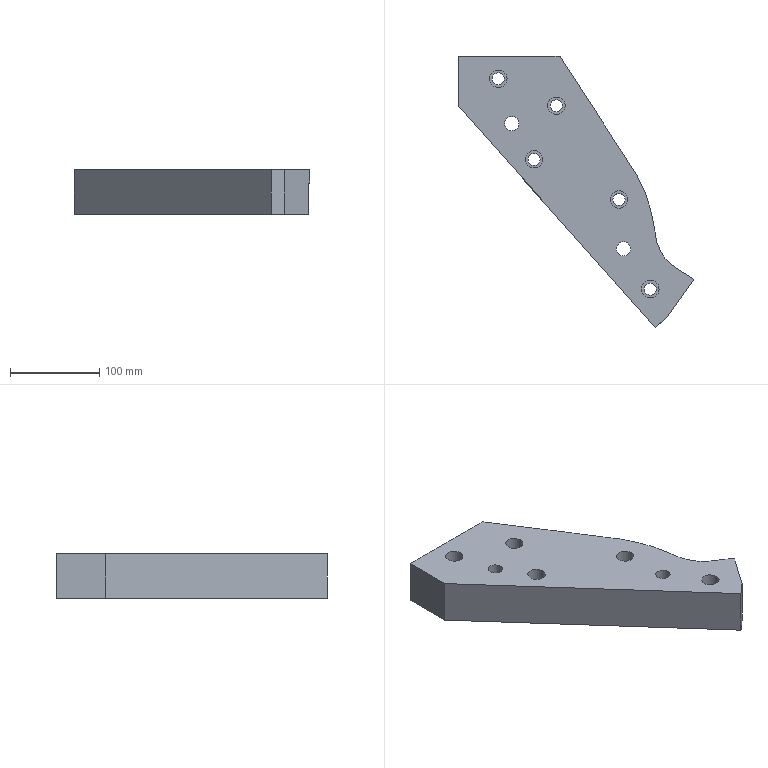Part | NX | features solid 2 | 1 solid | 29 faces | box 263.779 x 302.966 x 50 mm | volume 1530929 mm3 | plane 13 | cylinder 12 | spline 4 | commonest cylinder face diameters 13.5 x5 19.5 x5 16 x2
STEP:
#1=CARTESIAN_POINT('',(-697.,355.,0.));
#2=VERTEX_POINT('',#1);
#3=CARTESIAN_POINT('',(-705.,355.,0.));
#4=DIRECTION('',(0.,0.,1.));
#5=DIRECTION('',(1.,0.,0.));
#6=AXIS2_PLACEMENT_3D('',#3,#4,#5);
#7=CIRCLE('',#6,8.);
#8=EDGE_CURVE('',#2,#2,#7,.F.);
#9=ORIENTED_EDGE('',*,*,#8,.T.);
#10=EDGE_LOOP('',(#9));
#11=FACE_BOUND('',#10,.T.);
#12=CARTESIAN_POINT('',(-710.25,405.,0.));
#13=VERTEX_POINT('',#12);
#14=CARTESIAN_POINT('',(-720.,405.,0.));
#15=DIRECTION('',(0.,0.,1.));
#16=DIRECTION('',(1.,0.,0.));
#17=AXIS2_PLACEMENT_3D('',#14,#15,#16);
#18=CIRCLE('',#17,9.75);
#19=EDGE_CURVE('',#13,#13,#18,.F.);
#20=ORIENTED_EDGE('',*,*,#19,.T.);
#21=EDGE_LOOP('',(#20));
#22=FACE_BOUND('',#21,.T.);
#23=CARTESIAN_POINT('',(-575.25,270.,0.));
#24=VERTEX_POINT('',#23);
#25=CARTESIAN_POINT('',(-585.,270.,0.));
#26=DIRECTION('',(0.,0.,1.));
#27=DIRECTION('',(1.,0.,0.));
#28=AXIS2_PLACEMENT_3D('',#25,#26,#27);
#29=CIRCLE('',#28,9.75);
#30=EDGE_CURVE('',#24,#24,#29,.F.);
#31=ORIENTED_EDGE('',*,*,#30,.T.);
#32=EDGE_LOOP('',(#31));
#33=FACE_BOUND('',#32,.T.);
#34=CARTESIAN_POINT('',(-670.25,315.,0.));
#35=VERTEX_POINT('',#34);
#36=CARTESIAN_POINT('',(-680.,315.,0.));
#37=DIRECTION('',(0.,0.,1.));
#38=DIRECTION('',(1.,0.,0.));
#39=AXIS2_PLACEMENT_3D('',#36,#37,#38);
#40=CIRCLE('',#39,9.75);
#41=EDGE_CURVE('',#35,#35,#40,.F.);
#42=ORIENTED_EDGE('',*,*,#41,.T.);
#43=EDGE_LOOP('',(#42));
#44=FACE_BOUND('',#43,.T.);
#45=CARTESIAN_POINT('',(-546.519,244.221,0.));
#46=VERTEX_POINT('',#45);
#47=CARTESIAN_POINT('',(-650.95,430.,0.));
#48=VERTEX_POINT('',#47);
#49=CARTESIAN_POINT('',(-679.428,473.887,0.));
#50=CARTESIAN_POINT('',(-661.284,445.924,0.));
#51=CARTESIAN_POINT('',(-643.139,417.962,0.));
#52=CARTESIAN_POINT('',(-624.994,390.,0.));
#53=CARTESIAN_POINT('',(-607.333,362.782,0.));
#54=CARTESIAN_POINT('',(-589.671,335.563,0.));
#55=CARTESIAN_POINT('',(-572.009,308.345,0.));
#56=CARTESIAN_POINT('',(-559.323,288.796,0.));
#57=CARTESIAN_POINT('',(-549.988,267.187,0.));
#58=CARTESIAN_POINT('',(-546.519,244.221,0.));
#59=B_SPLINE_CURVE_WITH_KNOTS('',3,(#49,#50,#51,#52,#53,#54,#55,#56,#57,#58),.UNSPECIFIED.,.F.,.F.,(4,3,3,4),(0.,0.3747,0.7395,1.),.PIECEWISE_BEZIER_KNOTS.);
#60=EDGE_CURVE('',#46,#48,#59,.F.);
#61=ORIENTED_EDGE('',*,*,#60,.T.);
#62=CARTESIAN_POINT('',(-765.,430.,0.));
#63=VERTEX_POINT('',#62);
#64=CARTESIAN_POINT('',(-401.572,430.,0.));
#65=DIRECTION('',(-1.,0.,0.));
#66=VECTOR('',#65,1000.);
#67=LINE('',#64,#66);
#68=EDGE_CURVE('',#48,#63,#67,.T.);
#69=ORIENTED_EDGE('',*,*,#68,.T.);
#70=CARTESIAN_POINT('',(-765.,375.,0.));
#71=VERTEX_POINT('',#70);
#72=CARTESIAN_POINT('',(-765.,410.,0.));
#73=DIRECTION('',(0.,-1.,0.));
#74=VECTOR('',#73,1000.);
#75=LINE('',#72,#74);
#76=EDGE_CURVE('',#63,#71,#75,.T.);
#77=ORIENTED_EDGE('',*,*,#76,.T.);
#78=CARTESIAN_POINT('',(-544.586,127.034,0.));
#79=VERTEX_POINT('',#78);
#80=CARTESIAN_POINT('',(-406.474,-28.342,0.));
#81=DIRECTION('',(0.6644,-0.7474,0.));
#82=VECTOR('',#81,1000.);
#83=LINE('',#80,#82);
#84=EDGE_CURVE('',#71,#79,#83,.T.);
#85=ORIENTED_EDGE('',*,*,#84,.T.);
#86=CARTESIAN_POINT('',(-530.,140.,0.));
#87=VERTEX_POINT('',#86);
#88=CARTESIAN_POINT('',(-539.684,131.392,0.));
#89=DIRECTION('',(0.7474,0.6644,0.));
#90=VECTOR('',#89,1000.);
#91=LINE('',#88,#90);
#92=EDGE_CURVE('',#79,#87,#91,.T.);
#93=ORIENTED_EDGE('',*,*,#92,.T.);
#94=CARTESIAN_POINT('',(-501.221,181.1,0.));
#95=VERTEX_POINT('',#94);
#96=CARTESIAN_POINT('',(-564.796,90.306,0.));
#97=DIRECTION('',(-0.5736,-0.8192,0.));
#98=VECTOR('',#97,1000.);
#99=LINE('',#96,#98);
#100=EDGE_CURVE('',#95,#87,#99,.T.);
#101=ORIENTED_EDGE('',*,*,#100,.F.);
#102=CARTESIAN_POINT('',(-550.283,263.813,0.));
#103=CARTESIAN_POINT('',(-549.463,259.914,0.));
#104=CARTESIAN_POINT('',(-548.642,256.015,0.));
#105=CARTESIAN_POINT('',(-547.856,252.106,0.));
#106=CARTESIAN_POINT('',(-547.097,247.965,0.));
#107=CARTESIAN_POINT('',(-546.349,243.131,0.));
#108=CARTESIAN_POINT('',(-546.119,241.592,0.));
#109=CARTESIAN_POINT('',(-545.801,239.387,0.));
#110=CARTESIAN_POINT('',(-545.365,236.522,0.));
#111=CARTESIAN_POINT('',(-544.879,233.2,0.));
#112=CARTESIAN_POINT('',(-544.323,229.908,0.));
#113=CARTESIAN_POINT('',(-543.81,226.566,0.));
#114=CARTESIAN_POINT('',(-543.143,223.347,0.));
#115=CARTESIAN_POINT('',(-542.133,220.015,0.));
#116=CARTESIAN_POINT('',(-540.864,216.738,0.));
#117=CARTESIAN_POINT('',(-539.451,213.829,0.));
#118=CARTESIAN_POINT('',(-537.955,210.82,0.));
#119=CARTESIAN_POINT('',(-536.201,208.008,0.));
#120=CARTESIAN_POINT('',(-534.251,205.307,0.));
#121=CARTESIAN_POINT('',(-532.114,202.753,0.));
#122=CARTESIAN_POINT('',(-529.664,200.506,0.));
#123=CARTESIAN_POINT('',(-527.373,198.091,0.));
#124=CARTESIAN_POINT('',(-524.729,196.109,0.));
#125=CARTESIAN_POINT('',(-522.026,194.156,0.));
#126=CARTESIAN_POINT('',(-519.298,192.551,0.));
#127=CARTESIAN_POINT('',(-516.538,190.754,0.));
#128=CARTESIAN_POINT('',(-513.78,189.033,0.));
#129=CARTESIAN_POINT('',(-511.008,187.273,0.));
#130=CARTESIAN_POINT('',(-508.292,185.562,0.));
#131=CARTESIAN_POINT('',(-506.125,184.193,0.));
#132=CARTESIAN_POINT('',(-504.512,183.176,0.));
#133=CARTESIAN_POINT('',(-489.924,173.974,0.));
#134=CARTESIAN_POINT('',(-475.682,165.009,0.));
#135=CARTESIAN_POINT('',(-461.812,156.288,0.));
#136=CARTESIAN_POINT('',(-447.876,147.531,0.));
#137=CARTESIAN_POINT('',(-433.94,138.774,0.));
#138=B_SPLINE_CURVE_WITH_KNOTS('',5,(#102,#103,#104,#105,#106,#107,#108,#109,#110,#111,#112,#113,#114,#115,#116,#117,#118,#119,#120,#121,#122,#123,#124,#125,#126,#127,#128,#129,#130,#131,#132,#133,#134,#135,#136,#137),.UNSPECIFIED.,.F.,.F.,(6,3,1,1,1,1,1,1,1,1,1,1,1,1,1,1,1,1,1,1,1,1,1,1,1,1,3,6),(-0.2474,0.,0.01342,0.05471,0.09601,0.1373,0.1786,0.2199,0.2612,0.3025,0.3438,0.3851,0.4264,0.4677,0.509,0.5503,0.5916,0.6329,0.6742,0.7155,0.7568,0.7981,0.8394,0.8807,0.922,0.9633,1.,2.),.UNSPECIFIED.);
#139=EDGE_CURVE('',#95,#46,#138,.F.);
#140=ORIENTED_EDGE('',*,*,#139,.T.);
#141=EDGE_LOOP('',(#61,#69,#77,#85,#93,#101,#140));
#142=FACE_BOUND('',#141,.T.);
#143=CARTESIAN_POINT('',(-572.,215.,0.));
#144=VERTEX_POINT('',#143);
#145=CARTESIAN_POINT('',(-580.,215.,0.));
#146=DIRECTION('',(0.,0.,1.));
#147=DIRECTION('',(1.,0.,0.));
#148=AXIS2_PLACEMENT_3D('',#145,#146,#147);
#149=CIRCLE('',#148,8.);
#150=EDGE_CURVE('',#144,#144,#149,.F.);
#151=ORIENTED_EDGE('',*,*,#150,.T.);
#152=EDGE_LOOP('',(#151));
#153=FACE_BOUND('',#152,.T.);
#154=CARTESIAN_POINT('',(-540.25,170.,0.));
#155=VERTEX_POINT('',#154);
#156=CARTESIAN_POINT('',(-550.,170.,0.));
#157=DIRECTION('',(0.,0.,1.));
#158=DIRECTION('',(1.,0.,0.));
#159=AXIS2_PLACEMENT_3D('',#156,#157,#158);
#160=CIRCLE('',#159,9.75);
#161=EDGE_CURVE('',#155,#155,#160,.F.);
#162=ORIENTED_EDGE('',*,*,#161,.T.);
#163=EDGE_LOOP('',(#162));
#164=FACE_BOUND('',#163,.T.);
#165=CARTESIAN_POINT('',(-645.25,375.,0.));
#166=VERTEX_POINT('',#165);
#167=CARTESIAN_POINT('',(-655.,375.,0.));
#168=DIRECTION('',(0.,0.,1.));
#169=DIRECTION('',(1.,0.,0.));
#170=AXIS2_PLACEMENT_3D('',#167,#168,#169);
#171=CIRCLE('',#170,9.75);
#172=EDGE_CURVE('',#166,#166,#171,.F.);
#173=ORIENTED_EDGE('',*,*,#172,.T.);
#174=EDGE_LOOP('',(#173));
#175=FACE_BOUND('',#174,.T.);
#176=CARTESIAN_POINT('',(-401.572,-23.985,0.));
#177=DIRECTION('',(0.,0.,-1.));
#178=DIRECTION('',(-1.,0.,0.));
#179=AXIS2_PLACEMENT_3D('',#176,#177,#178);
#180=PLANE('',#179);
#181=ADVANCED_FACE('',(#11,#22,#33,#44,#142,#153,#164,#175),#180,.F.);
#182=CARTESIAN_POINT('',(-648.25,375.,-50.));
#183=VERTEX_POINT('',#182);
#184=CARTESIAN_POINT('',(-655.,375.,-50.));
#185=DIRECTION('',(0.,0.,1.));
#186=DIRECTION('',(1.,0.,0.));
#187=AXIS2_PLACEMENT_3D('',#184,#185,#186);
#188=CIRCLE('',#187,6.75);
#189=EDGE_CURVE('',#183,#183,#188,.F.);
#190=ORIENTED_EDGE('',*,*,#189,.T.);
#191=EDGE_LOOP('',(#190));
#192=FACE_BOUND('',#191,.T.);
#193=CARTESIAN_POINT('',(-661.75,375.,-25.));
#194=VERTEX_POINT('',#193);
#195=CARTESIAN_POINT('',(-655.,375.,-25.));
#196=DIRECTION('',(0.,0.,-1.));
#197=DIRECTION('',(-1.,0.,0.));
#198=AXIS2_PLACEMENT_3D('',#195,#196,#197);
#199=CIRCLE('',#198,6.75);
#200=EDGE_CURVE('',#194,#194,#199,.T.);
#201=ORIENTED_EDGE('',*,*,#200,.F.);
#202=EDGE_LOOP('',(#201));
#203=FACE_BOUND('',#202,.T.);
#204=CARTESIAN_POINT('',(-655.,375.,175.));
#205=DIRECTION('',(0.,0.,-1.));
#206=DIRECTION('',(1.,0.,0.));
#207=AXIS2_PLACEMENT_3D('',#204,#205,#206);
#208=CYLINDRICAL_SURFACE('',#207,6.75);
#209=ADVANCED_FACE('',(#192,#203),#208,.F.);
#210=CARTESIAN_POINT('',(-572.,215.,-50.));
#211=VERTEX_POINT('',#210);
#212=CARTESIAN_POINT('',(-580.,215.,-50.));
#213=DIRECTION('',(0.,0.,1.));
#214=DIRECTION('',(1.,0.,0.));
#215=AXIS2_PLACEMENT_3D('',#212,#213,#214);
#216=CIRCLE('',#215,8.);
#217=EDGE_CURVE('',#211,#211,#216,.F.);
#218=ORIENTED_EDGE('',*,*,#217,.F.);
#219=EDGE_LOOP('',(#218));
#220=FACE_BOUND('',#219,.T.);
#221=CARTESIAN_POINT('',(-543.25,170.,-50.));
#222=VERTEX_POINT('',#221);
#223=CARTESIAN_POINT('',(-550.,170.,-50.));
#224=DIRECTION('',(0.,0.,1.));
#225=DIRECTION('',(1.,0.,0.));
#226=AXIS2_PLACEMENT_3D('',#223,#224,#225);
#227=CIRCLE('',#226,6.75);
#228=EDGE_CURVE('',#222,#222,#227,.F.);
#229=ORIENTED_EDGE('',*,*,#228,.F.);
#230=EDGE_LOOP('',(#229));
#231=FACE_BOUND('',#230,.T.);
#232=CARTESIAN_POINT('',(-697.,355.,-50.));
#233=VERTEX_POINT('',#232);
#234=CARTESIAN_POINT('',(-705.,355.,-50.));
#235=DIRECTION('',(0.,0.,1.));
#236=DIRECTION('',(1.,0.,0.));
#237=AXIS2_PLACEMENT_3D('',#234,#235,#236);
#238=CIRCLE('',#237,8.);
#239=EDGE_CURVE('',#233,#233,#238,.F.);
#240=ORIENTED_EDGE('',*,*,#239,.F.);
#241=EDGE_LOOP('',(#240));
#242=FACE_BOUND('',#241,.T.);
#243=CARTESIAN_POINT('',(-713.25,405.,-50.));
#244=VERTEX_POINT('',#243);
#245=CARTESIAN_POINT('',(-720.,405.,-50.));
#246=DIRECTION('',(0.,0.,1.));
#247=DIRECTION('',(1.,0.,0.));
#248=AXIS2_PLACEMENT_3D('',#245,#246,#247);
#249=CIRCLE('',#248,6.75);
#250=EDGE_CURVE('',#244,#244,#249,.F.);
#251=ORIENTED_EDGE('',*,*,#250,.F.);
#252=EDGE_LOOP('',(#251));
#253=FACE_BOUND('',#252,.T.);
#254=CARTESIAN_POINT('',(-578.25,270.,-50.));
#255=VERTEX_POINT('',#254);
#256=CARTESIAN_POINT('',(-585.,270.,-50.));
#257=DIRECTION('',(0.,0.,1.));
#258=DIRECTION('',(1.,0.,0.));
#259=AXIS2_PLACEMENT_3D('',#256,#257,#258);
#260=CIRCLE('',#259,6.75);
#261=EDGE_CURVE('',#255,#255,#260,.F.);
#262=ORIENTED_EDGE('',*,*,#261,.F.);
#263=EDGE_LOOP('',(#262));
#264=FACE_BOUND('',#263,.T.);
#265=CARTESIAN_POINT('',(-673.25,315.,-50.));
#266=VERTEX_POINT('',#265);
#267=CARTESIAN_POINT('',(-680.,315.,-50.));
#268=DIRECTION('',(0.,0.,1.));
#269=DIRECTION('',(1.,0.,0.));
#270=AXIS2_PLACEMENT_3D('',#267,#268,#269);
#271=CIRCLE('',#270,6.75);
#272=EDGE_CURVE('',#266,#266,#271,.F.);
#273=ORIENTED_EDGE('',*,*,#272,.F.);
#274=EDGE_LOOP('',(#273));
#275=FACE_BOUND('',#274,.T.);
#276=CARTESIAN_POINT('',(-765.,375.,-50.));
#277=VERTEX_POINT('',#276);
#278=CARTESIAN_POINT('',(-544.586,127.034,-50.));
#279=VERTEX_POINT('',#278);
#280=CARTESIAN_POINT('',(-406.474,-28.342,-50.));
#281=DIRECTION('',(0.6644,-0.7474,0.));
#282=VECTOR('',#281,1000.);
#283=LINE('',#280,#282);
#284=EDGE_CURVE('',#277,#279,#283,.T.);
#285=ORIENTED_EDGE('',*,*,#284,.F.);
#286=CARTESIAN_POINT('',(-765.,430.,-50.));
#287=VERTEX_POINT('',#286);
#288=CARTESIAN_POINT('',(-765.,410.,-50.));
#289=DIRECTION('',(0.,-1.,0.));
#290=VECTOR('',#289,1000.);
#291=LINE('',#288,#290);
#292=EDGE_CURVE('',#287,#277,#291,.T.);
#293=ORIENTED_EDGE('',*,*,#292,.F.);
#294=CARTESIAN_POINT('',(-653.334,430.,-50.));
#295=VERTEX_POINT('',#294);
#296=CARTESIAN_POINT('',(-401.572,430.,-50.));
#297=DIRECTION('',(-1.,0.,0.));
#298=VECTOR('',#297,1000.);
#299=LINE('',#296,#298);
#300=EDGE_CURVE('',#295,#287,#299,.T.);
#301=ORIENTED_EDGE('',*,*,#300,.F.);
#302=CARTESIAN_POINT('',(-637.001,404.828,-50.));
#303=VERTEX_POINT('',#302);
#304=CARTESIAN_POINT('',(-637.001,404.828,-50.));
#305=CARTESIAN_POINT('',(-642.445,413.219,-50.));
#306=CARTESIAN_POINT('',(-647.89,421.609,-50.));
#307=CARTESIAN_POINT('',(-653.334,430.,-50.));
#308=B_SPLINE_CURVE_WITH_KNOTS('',3,(#304,#305,#306,#307),.UNSPECIFIED.,.F.,.F.,(4,4),(0.05984,0.08984),.UNSPECIFIED.);
#309=EDGE_CURVE('',#303,#295,#308,.T.);
#310=ORIENTED_EDGE('',*,*,#309,.F.);
#311=CARTESIAN_POINT('',(-548.499,243.922,-50.));
#312=VERTEX_POINT('',#311);
#313=CARTESIAN_POINT('',(-548.497,243.922,-50.));
#314=CARTESIAN_POINT('',(-549.657,251.602,-50.));
#315=CARTESIAN_POINT('',(-553.279,266.514,-50.));
#316=CARTESIAN_POINT('',(-560.547,284.175,-50.));
#317=CARTESIAN_POINT('',(-567.793,297.855,-50.));
#318=CARTESIAN_POINT('',(-573.914,307.693,-50.));
#319=CARTESIAN_POINT('',(-580.268,317.377,-50.));
#320=CARTESIAN_POINT('',(-588.658,330.342,-50.));
#321=CARTESIAN_POINT('',(-599.174,346.53,-50.));
#322=CARTESIAN_POINT('',(-615.984,372.442,-50.));
#323=CARTESIAN_POINT('',(-628.594,391.874,-50.));
#324=CARTESIAN_POINT('',(-637.001,404.828,-50.));
#325=B_SPLINE_CURVE_WITH_KNOTS('',3,(#313,#314,#315,#316,#317,#318,#319,#320,#321,#322,#323,#324),.UNSPECIFIED.,.F.,.F.,(4,1,1,1,1,1,1,1,1,4),(0.8596,0.8829,0.9062,0.9179,0.9295,0.9412,0.9528,0.9761,0.9994,1.046),.UNSPECIFIED.);
#326=EDGE_CURVE('',#312,#303,#325,.T.);
#327=ORIENTED_EDGE('',*,*,#326,.F.);
#328=CARTESIAN_POINT('',(-504.108,180.556,-50.));
#329=VERTEX_POINT('',#328);
#330=CARTESIAN_POINT('',(-504.108,180.556,-50.));
#331=CARTESIAN_POINT('',(-504.118,180.563,-50.));
#332=CARTESIAN_POINT('',(-504.647,180.896,-50.));
#333=CARTESIAN_POINT('',(-506.377,181.988,-50.));
#334=CARTESIAN_POINT('',(-508.187,183.131,-50.));
#335=CARTESIAN_POINT('',(-510.51,184.596,-50.));
#336=CARTESIAN_POINT('',(-512.872,186.087,-50.));
#337=CARTESIAN_POINT('',(-515.019,187.442,-50.));
#338=CARTESIAN_POINT('',(-516.756,188.538,-50.));
#339=CARTESIAN_POINT('',(-518.313,189.521,-50.));
#340=CARTESIAN_POINT('',(-519.617,190.344,-50.));
#341=CARTESIAN_POINT('',(-520.473,190.884,-50.));
#342=CARTESIAN_POINT('',(-521.14,191.305,-50.));
#343=CARTESIAN_POINT('',(-521.741,191.685,-50.));
#344=CARTESIAN_POINT('',(-521.993,191.844,-50.));
#345=CARTESIAN_POINT('',(-522.378,192.09,-50.));
#346=CARTESIAN_POINT('',(-522.834,192.385,-50.));
#347=CARTESIAN_POINT('',(-523.557,192.863,-50.));
#348=CARTESIAN_POINT('',(-524.429,193.457,-50.));
#349=CARTESIAN_POINT('',(-525.424,194.164,-50.));
#350=CARTESIAN_POINT('',(-526.391,194.879,-50.));
#351=CARTESIAN_POINT('',(-527.408,195.679,-50.));
#352=CARTESIAN_POINT('',(-528.38,196.494,-50.));
#353=CARTESIAN_POINT('',(-529.161,197.188,-50.));
#354=CARTESIAN_POINT('',(-529.718,197.708,-50.));
#355=CARTESIAN_POINT('',(-529.996,197.973,-50.));
#356=CARTESIAN_POINT('',(-530.41,198.373,-50.));
#357=CARTESIAN_POINT('',(-530.897,198.844,-50.));
#358=CARTESIAN_POINT('',(-531.621,199.553,-50.));
#359=CARTESIAN_POINT('',(-532.421,200.347,-50.));
#360=CARTESIAN_POINT('',(-533.077,201.014,-50.));
#361=CARTESIAN_POINT('',(-533.527,201.485,-50.));
#362=CARTESIAN_POINT('',(-533.794,201.771,-50.));
#363=CARTESIAN_POINT('',(-534.23,202.253,-50.));
#364=CARTESIAN_POINT('',(-535.012,203.151,-50.));
#365=CARTESIAN_POINT('',(-535.937,204.298,-50.));
#366=CARTESIAN_POINT('',(-537.002,205.749,-50.));
#367=CARTESIAN_POINT('',(-537.95,207.118,-50.));
#368=CARTESIAN_POINT('',(-539.548,209.637,-50.));
#369=CARTESIAN_POINT('',(-541.113,212.639,-50.));
#370=CARTESIAN_POINT('',(-542.572,215.784,-50.));
#371=CARTESIAN_POINT('',(-543.551,218.208,-50.));
#372=CARTESIAN_POINT('',(-544.378,220.606,-50.));
#373=CARTESIAN_POINT('',(-544.957,222.647,-50.));
#374=CARTESIAN_POINT('',(-545.285,224.003,-50.));
#375=CARTESIAN_POINT('',(-545.477,224.892,-50.));
#376=CARTESIAN_POINT('',(-545.571,225.354,-50.));
#377=CARTESIAN_POINT('',(-545.704,226.039,-50.));
#378=CARTESIAN_POINT('',(-545.935,227.312,-50.));
#379=CARTESIAN_POINT('',(-546.266,229.254,-50.));
#380=CARTESIAN_POINT('',(-546.654,231.683,-50.));
#381=CARTESIAN_POINT('',(-546.991,233.869,-50.));
#382=CARTESIAN_POINT('',(-547.276,235.754,-50.));
#383=CARTESIAN_POINT('',(-547.476,237.092,-50.));
#384=CARTESIAN_POINT('',(-547.638,238.176,-50.));
#385=CARTESIAN_POINT('',(-547.755,238.962,-50.));
#386=CARTESIAN_POINT('',(-547.82,239.402,-50.));
#387=CARTESIAN_POINT('',(-547.878,239.792,-50.));
#388=CARTESIAN_POINT('',(-547.972,240.428,-50.));
#389=CARTESIAN_POINT('',(-548.112,241.372,-50.));
#390=CARTESIAN_POINT('',(-548.305,242.654,-50.));
#391=CARTESIAN_POINT('',(-548.438,243.521,-50.));
#392=CARTESIAN_POINT('',(-548.501,243.921,-50.));
#393=B_SPLINE_CURVE_WITH_KNOTS('',3,(#330,#331,#332,#333,#334,#335,#336,#337,#338,#339,#340,#341,#342,#343,#344,#345,#346,#347,#348,#349,#350,#351,#352,#353,#354,#355,#356,#357,#358,#359,#360,#361,#362,#363,#364,#365,#366,#367,#368,#369,#370,#371,#372,#373,#374,#375,#376,#377,#378,#379,#380,#381,#382,#383,#384,#385,#386,#387,#388,#389,#390,#391,#392),.UNSPECIFIED.,.F.,.F.,(4,1,1,1,1,1,1,1,1,1,1,1,1,1,1,1,1,1,1,1,1,1,1,1,1,1,1,1,1,1,1,1,1,1,1,1,1,1,1,1,1,1,1,1,1,1,1,1,1,1,1,1,1,1,1,1,1,1,1,1,4),(0.,0.01512,0.02268,0.03024,0.0378,0.04536,0.04914,0.05292,0.0567,0.05859,0.06048,0.06143,0.06237,0.06332,0.06426,0.06615,0.06804,0.07183,0.07561,0.07939,0.08317,0.08695,0.09073,0.09262,0.09356,0.09451,0.0964,0.09829,0.1021,0.1058,0.1077,0.1096,0.1115,0.1134,0.121,0.1247,0.1285,0.1361,0.1512,0.1588,0.1663,0.1739,0.1815,0.1852,0.1871,0.189,0.1928,0.1966,0.2041,0.2117,0.2155,0.2193,0.223,0.2268,0.2287,0.2306,0.2315,0.2325,0.2344,0.2382,0.2419),.UNSPECIFIED.);
#394=EDGE_CURVE('',#329,#312,#393,.T.);
#395=ORIENTED_EDGE('',*,*,#394,.F.);
#396=CARTESIAN_POINT('',(-502.37,179.46,-50.));
#397=VERTEX_POINT('',#396);
#398=CARTESIAN_POINT('',(-502.37,179.46,-50.));
#399=CARTESIAN_POINT('',(-502.949,179.825,-50.));
#400=CARTESIAN_POINT('',(-503.528,180.191,-50.));
#401=CARTESIAN_POINT('',(-504.108,180.556,-50.));
#402=B_SPLINE_CURVE_WITH_KNOTS('',3,(#398,#399,#400,#401),.UNSPECIFIED.,.F.,.F.,(4,4),(0.,0.002055),.UNSPECIFIED.);
#403=EDGE_CURVE('',#397,#329,#402,.T.);
#404=ORIENTED_EDGE('',*,*,#403,.F.);
#405=CARTESIAN_POINT('',(-530.,140.,-50.));
#406=VERTEX_POINT('',#405);
#407=CARTESIAN_POINT('',(-564.796,90.306,-50.));
#408=DIRECTION('',(0.5736,0.8192,0.));
#409=VECTOR('',#408,1000.);
#410=LINE('',#407,#409);
#411=EDGE_CURVE('',#406,#397,#410,.T.);
#412=ORIENTED_EDGE('',*,*,#411,.F.);
#413=CARTESIAN_POINT('',(-539.684,131.392,-50.));
#414=DIRECTION('',(0.7474,0.6644,0.));
#415=VECTOR('',#414,1000.);
#416=LINE('',#413,#415);
#417=EDGE_CURVE('',#279,#406,#416,.T.);
#418=ORIENTED_EDGE('',*,*,#417,.F.);
#419=EDGE_LOOP('',(#285,#293,#301,#310,#327,#395,#404,#412,#418));
#420=FACE_BOUND('',#419,.T.);
#421=ORIENTED_EDGE('',*,*,#189,.F.);
#422=EDGE_LOOP('',(#421));
#423=FACE_BOUND('',#422,.T.);
#424=CARTESIAN_POINT('',(-401.572,-23.985,-50.));
#425=DIRECTION('',(0.,0.,-1.));
#426=DIRECTION('',(-1.,0.,0.));
#427=AXIS2_PLACEMENT_3D('',#424,#425,#426);
#428=PLANE('',#427);
#429=ADVANCED_FACE('',(#220,#231,#242,#253,#264,#275,#420,#423),#428,.T.);
#430=CARTESIAN_POINT('',(-653.334,430.,-15.));
#431=VERTEX_POINT('',#430);
#432=CARTESIAN_POINT('',(-548.497,243.922,-15.));
#433=VERTEX_POINT('',#432);
#434=CARTESIAN_POINT('',(-653.334,430.,-15.));
#435=CARTESIAN_POINT('',(-648.462,422.491,-15.));
#436=CARTESIAN_POINT('',(-638.716,407.472,-15.));
#437=CARTESIAN_POINT('',(-624.097,384.943,-15.));
#438=CARTESIAN_POINT('',(-609.478,362.415,-15.));
#439=CARTESIAN_POINT('',(-594.863,339.885,-15.));
#440=CARTESIAN_POINT('',(-583.888,322.994,-15.));
#441=CARTESIAN_POINT('',(-576.593,311.722,-15.));
#442=CARTESIAN_POINT('',(-571.679,304.234,-15.));
#443=CARTESIAN_POINT('',(-565.97,294.657,-15.));
#444=CARTESIAN_POINT('',(-560.006,282.72,-15.));
#445=CARTESIAN_POINT('',(-554.983,270.325,-15.));
#446=CARTESIAN_POINT('',(-551.006,257.374,-15.));
#447=CARTESIAN_POINT('',(-549.176,248.416,-15.));
#448=CARTESIAN_POINT('',(-548.497,243.922,-15.));
#449=B_SPLINE_CURVE_WITH_KNOTS('',3,(#434,#435,#436,#437,#438,#439,#440,#441,#442,#443,#444,#445,#446,#447,#448),.UNSPECIFIED.,.F.,.F.,(4,1,1,1,1,1,1,1,1,1,1,1,4),(0.07118,0.09803,0.1249,0.1517,0.1786,0.2055,0.2122,0.2189,0.2323,0.2457,0.2592,0.2726,0.286),.UNSPECIFIED.);
#450=EDGE_CURVE('',#431,#433,#449,.T.);
#451=ORIENTED_EDGE('',*,*,#450,.F.);
#452=CARTESIAN_POINT('',(-650.95,430.,-15.));
#453=VERTEX_POINT('',#452);
#454=CARTESIAN_POINT('',(-667.419,430.,-15.));
#455=DIRECTION('',(-1.,0.,0.));
#456=VECTOR('',#455,1000.);
#457=LINE('',#454,#456);
#458=EDGE_CURVE('',#453,#431,#457,.T.);
#459=ORIENTED_EDGE('',*,*,#458,.F.);
#460=CARTESIAN_POINT('',(-546.519,244.221,-15.));
#461=VERTEX_POINT('',#460);
#462=CARTESIAN_POINT('',(-679.428,473.887,-15.));
#463=CARTESIAN_POINT('',(-661.284,445.924,-15.));
#464=CARTESIAN_POINT('',(-643.139,417.962,-15.));
#465=CARTESIAN_POINT('',(-624.994,390.,-15.));
#466=CARTESIAN_POINT('',(-607.333,362.782,-15.));
#467=CARTESIAN_POINT('',(-589.671,335.563,-15.));
#468=CARTESIAN_POINT('',(-572.009,308.345,-15.));
#469=CARTESIAN_POINT('',(-559.323,288.796,-15.));
#470=CARTESIAN_POINT('',(-549.988,267.187,-15.));
#471=CARTESIAN_POINT('',(-546.519,244.221,-15.));
#472=B_SPLINE_CURVE_WITH_KNOTS('',3,(#462,#463,#464,#465,#466,#467,#468,#469,#470,#471),.UNSPECIFIED.,.F.,.F.,(4,3,3,4),(0.,0.3747,0.7395,1.),.PIECEWISE_BEZIER_KNOTS.);
#473=EDGE_CURVE('',#461,#453,#472,.F.);
#474=ORIENTED_EDGE('',*,*,#473,.F.);
#475=CARTESIAN_POINT('',(-501.221,181.1,-15.));
#476=VERTEX_POINT('',#475);
#477=CARTESIAN_POINT('',(-550.283,263.813,-15.));
#478=CARTESIAN_POINT('',(-549.463,259.914,-15.));
#479=CARTESIAN_POINT('',(-548.642,256.015,-15.));
#480=CARTESIAN_POINT('',(-547.856,252.106,-15.));
#481=CARTESIAN_POINT('',(-547.097,247.965,-15.));
#482=CARTESIAN_POINT('',(-546.349,243.131,-15.));
#483=CARTESIAN_POINT('',(-546.119,241.592,-15.));
#484=CARTESIAN_POINT('',(-545.801,239.387,-15.));
#485=CARTESIAN_POINT('',(-545.365,236.522,-15.));
#486=CARTESIAN_POINT('',(-544.879,233.2,-15.));
#487=CARTESIAN_POINT('',(-544.323,229.908,-15.));
#488=CARTESIAN_POINT('',(-543.81,226.566,-15.));
#489=CARTESIAN_POINT('',(-543.143,223.347,-15.));
#490=CARTESIAN_POINT('',(-542.133,220.015,-15.));
#491=CARTESIAN_POINT('',(-540.864,216.738,-15.));
#492=CARTESIAN_POINT('',(-539.451,213.829,-15.));
#493=CARTESIAN_POINT('',(-537.955,210.82,-15.));
#494=CARTESIAN_POINT('',(-536.201,208.008,-15.));
#495=CARTESIAN_POINT('',(-534.251,205.307,-15.));
#496=CARTESIAN_POINT('',(-532.114,202.753,-15.));
#497=CARTESIAN_POINT('',(-529.664,200.506,-15.));
#498=CARTESIAN_POINT('',(-527.373,198.091,-15.));
#499=CARTESIAN_POINT('',(-524.729,196.109,-15.));
#500=CARTESIAN_POINT('',(-522.026,194.156,-15.));
#501=CARTESIAN_POINT('',(-519.298,192.551,-15.));
#502=CARTESIAN_POINT('',(-516.538,190.754,-15.));
#503=CARTESIAN_POINT('',(-513.78,189.033,-15.));
#504=CARTESIAN_POINT('',(-511.008,187.273,-15.));
#505=CARTESIAN_POINT('',(-508.292,185.562,-15.));
#506=CARTESIAN_POINT('',(-506.125,184.193,-15.));
#507=CARTESIAN_POINT('',(-504.512,183.176,-15.));
#508=CARTESIAN_POINT('',(-489.924,173.974,-15.));
#509=CARTESIAN_POINT('',(-475.682,165.009,-15.));
#510=CARTESIAN_POINT('',(-461.812,156.288,-15.));
#511=CARTESIAN_POINT('',(-447.876,147.531,-15.));
#512=CARTESIAN_POINT('',(-433.94,138.774,-15.));
#513=B_SPLINE_CURVE_WITH_KNOTS('',5,(#477,#478,#479,#480,#481,#482,#483,#484,#485,#486,#487,#488,#489,#490,#491,#492,#493,#494,#495,#496,#497,#498,#499,#500,#501,#502,#503,#504,#505,#506,#507,#508,#509,#510,#511,#512),.UNSPECIFIED.,.F.,.F.,(6,3,1,1,1,1,1,1,1,1,1,1,1,1,1,1,1,1,1,1,1,1,1,1,1,1,3,6),(-0.2474,0.,0.01342,0.05471,0.09601,0.1373,0.1786,0.2199,0.2612,0.3025,0.3438,0.3851,0.4264,0.4677,0.509,0.5503,0.5916,0.6329,0.6742,0.7155,0.7568,0.7981,0.8394,0.8807,0.922,0.9633,1.,2.),.UNSPECIFIED.);
#514=EDGE_CURVE('',#476,#461,#513,.F.);
#515=ORIENTED_EDGE('',*,*,#514,.F.);
#516=CARTESIAN_POINT('',(-502.37,179.46,-15.));
#517=VERTEX_POINT('',#516);
#518=CARTESIAN_POINT('',(-457.472,243.58,-15.));
#519=DIRECTION('',(-0.5736,-0.8192,0.));
#520=VECTOR('',#519,1000.);
#521=LINE('',#518,#520);
#522=EDGE_CURVE('',#476,#517,#521,.T.);
#523=ORIENTED_EDGE('',*,*,#522,.T.);
#524=CARTESIAN_POINT('',(-502.37,179.46,-15.));
#525=CARTESIAN_POINT('',(-505.335,181.33,-15.));
#526=CARTESIAN_POINT('',(-511.265,185.067,-15.));
#527=CARTESIAN_POINT('',(-518.665,189.758,-15.));
#528=CARTESIAN_POINT('',(-524.602,193.486,-15.));
#529=CARTESIAN_POINT('',(-528.09,196.134,-15.));
#530=CARTESIAN_POINT('',(-530.639,198.594,-15.));
#531=CARTESIAN_POINT('',(-532.545,200.454,-15.));
#532=CARTESIAN_POINT('',(-534.388,202.381,-15.));
#533=CARTESIAN_POINT('',(-536.597,205.108,-15.));
#534=CARTESIAN_POINT('',(-539.066,208.712,-15.));
#535=CARTESIAN_POINT('',(-541.508,213.388,-15.));
#536=CARTESIAN_POINT('',(-543.647,218.24,-15.));
#537=CARTESIAN_POINT('',(-545.209,223.22,-15.));
#538=CARTESIAN_POINT('',(-546.123,228.372,-15.));
#539=CARTESIAN_POINT('',(-547.229,235.268,-15.));
#540=CARTESIAN_POINT('',(-547.953,240.472,-15.));
#541=CARTESIAN_POINT('',(-548.497,243.922,-15.));
#542=B_SPLINE_CURVE_WITH_KNOTS('',3,(#524,#525,#526,#527,#528,#529,#530,#531,#532,#533,#534,#535,#536,#537,#538,#539,#540,#541),.UNSPECIFIED.,.F.,.F.,(4,1,1,1,1,1,1,1,1,1,1,1,1,1,1,4),(0.3461,0.3567,0.3672,0.3724,0.3777,0.3803,0.3829,0.3856,0.3882,0.3935,0.3987,0.404,0.4092,0.4145,0.4197,0.4303),.UNSPECIFIED.);
#543=EDGE_CURVE('',#433,#517,#542,.F.);
#544=ORIENTED_EDGE('',*,*,#543,.F.);
#545=EDGE_LOOP('',(#451,#459,#474,#515,#523,#544));
#546=FACE_BOUND('',#545,.T.);
#547=CARTESIAN_POINT('',(-667.419,390.587,-15.));
#548=DIRECTION('',(0.,0.,-1.));
#549=DIRECTION('',(-0.08716,0.9962,0.));
#550=AXIS2_PLACEMENT_3D('',#547,#548,#549);
#551=PLANE('',#550);
#552=ADVANCED_FACE('',(#546),#551,.T.);
#553=ORIENTED_EDGE('',*,*,#458,.T.);
#554=CARTESIAN_POINT('',(-653.334,430.,-32.5));
#555=DIRECTION('',(0.,0.,-1.));
#556=VECTOR('',#555,1000.);
#557=LINE('',#554,#556);
#558=EDGE_CURVE('',#295,#431,#557,.F.);
#559=ORIENTED_EDGE('',*,*,#558,.F.);
#560=ORIENTED_EDGE('',*,*,#300,.T.);
#561=CARTESIAN_POINT('',(-765.,430.,-50.));
#562=DIRECTION('',(0.,0.,1.));
#563=VECTOR('',#562,1000.);
#564=LINE('',#561,#563);
#565=EDGE_CURVE('',#287,#63,#564,.T.);
#566=ORIENTED_EDGE('',*,*,#565,.T.);
#567=ORIENTED_EDGE('',*,*,#68,.F.);
#568=CARTESIAN_POINT('',(-650.95,430.,-200.));
#569=DIRECTION('',(0.,0.,1.));
#570=VECTOR('',#569,1000.);
#571=LINE('',#568,#570);
#572=EDGE_CURVE('',#453,#48,#571,.T.);
#573=ORIENTED_EDGE('',*,*,#572,.F.);
#574=EDGE_LOOP('',(#553,#559,#560,#566,#567,#573));
#575=FACE_BOUND('',#574,.T.);
#576=CARTESIAN_POINT('',(-752.827,430.,-50.));
#577=DIRECTION('',(0.,1.,0.));
#578=DIRECTION('',(-1.,0.,0.));
#579=AXIS2_PLACEMENT_3D('',#576,#577,#578);
#580=PLANE('',#579);
#581=ADVANCED_FACE('',(#575),#580,.T.);
#582=ORIENTED_EDGE('',*,*,#250,.T.);
#583=EDGE_LOOP('',(#582));
#584=FACE_BOUND('',#583,.T.);
#585=CARTESIAN_POINT('',(-726.75,405.,-25.));
#586=VERTEX_POINT('',#585);
#587=CARTESIAN_POINT('',(-720.,405.,-25.));
#588=DIRECTION('',(0.,0.,-1.));
#589=DIRECTION('',(-1.,0.,0.));
#590=AXIS2_PLACEMENT_3D('',#587,#588,#589);
#591=CIRCLE('',#590,6.75);
#592=EDGE_CURVE('',#586,#586,#591,.T.);
#593=ORIENTED_EDGE('',*,*,#592,.F.);
#594=EDGE_LOOP('',(#593));
#595=FACE_BOUND('',#594,.T.);
#596=CARTESIAN_POINT('',(-720.,405.,75.));
#597=DIRECTION('',(0.,0.,-1.));
#598=DIRECTION('',(1.,0.,0.));
#599=AXIS2_PLACEMENT_3D('',#596,#597,#598);
#600=CYLINDRICAL_SURFACE('',#599,6.75);
#601=ADVANCED_FACE('',(#584,#595),#600,.F.);
#602=ORIENTED_EDGE('',*,*,#272,.T.);
#603=EDGE_LOOP('',(#602));
#604=FACE_BOUND('',#603,.T.);
#605=CARTESIAN_POINT('',(-686.75,315.,-25.));
#606=VERTEX_POINT('',#605);
#607=CARTESIAN_POINT('',(-680.,315.,-25.));
#608=DIRECTION('',(0.,0.,-1.));
#609=DIRECTION('',(-1.,0.,0.));
#610=AXIS2_PLACEMENT_3D('',#607,#608,#609);
#611=CIRCLE('',#610,6.75);
#612=EDGE_CURVE('',#606,#606,#611,.T.);
#613=ORIENTED_EDGE('',*,*,#612,.F.);
#614=EDGE_LOOP('',(#613));
#615=FACE_BOUND('',#614,.T.);
#616=CARTESIAN_POINT('',(-680.,315.,75.));
#617=DIRECTION('',(0.,0.,-1.));
#618=DIRECTION('',(1.,0.,0.));
#619=AXIS2_PLACEMENT_3D('',#616,#617,#618);
#620=CYLINDRICAL_SURFACE('',#619,6.75);
#621=ADVANCED_FACE('',(#604,#615),#620,.F.);
#622=ORIENTED_EDGE('',*,*,#261,.T.);
#623=EDGE_LOOP('',(#622));
#624=FACE_BOUND('',#623,.T.);
#625=CARTESIAN_POINT('',(-591.75,270.,-25.));
#626=VERTEX_POINT('',#625);
#627=CARTESIAN_POINT('',(-585.,270.,-25.));
#628=DIRECTION('',(0.,0.,-1.));
#629=DIRECTION('',(-1.,0.,0.));
#630=AXIS2_PLACEMENT_3D('',#627,#628,#629);
#631=CIRCLE('',#630,6.75);
#632=EDGE_CURVE('',#626,#626,#631,.T.);
#633=ORIENTED_EDGE('',*,*,#632,.F.);
#634=EDGE_LOOP('',(#633));
#635=FACE_BOUND('',#634,.T.);
#636=CARTESIAN_POINT('',(-585.,270.,75.));
#637=DIRECTION('',(0.,0.,-1.));
#638=DIRECTION('',(1.,0.,0.));
#639=AXIS2_PLACEMENT_3D('',#636,#637,#638);
#640=CYLINDRICAL_SURFACE('',#639,6.75);
#641=ADVANCED_FACE('',(#624,#635),#640,.F.);
#642=CARTESIAN_POINT('',(-765.,375.,-50.));
#643=DIRECTION('',(0.,0.,-1.));
#644=VECTOR('',#643,1000.);
#645=LINE('',#642,#644);
#646=EDGE_CURVE('',#71,#277,#645,.T.);
#647=ORIENTED_EDGE('',*,*,#646,.F.);
#648=ORIENTED_EDGE('',*,*,#76,.F.);
#649=ORIENTED_EDGE('',*,*,#565,.F.);
#650=ORIENTED_EDGE('',*,*,#292,.T.);
#651=EDGE_LOOP('',(#647,#648,#649,#650));
#652=FACE_BOUND('',#651,.T.);
#653=CARTESIAN_POINT('',(-765.,410.,-50.));
#654=DIRECTION('',(-1.,0.,0.));
#655=DIRECTION('',(0.,-1.,0.));
#656=AXIS2_PLACEMENT_3D('',#653,#654,#655);
#657=PLANE('',#656);
#658=ADVANCED_FACE('',(#652),#657,.T.);
#659=ORIENTED_EDGE('',*,*,#84,.F.);
#660=ORIENTED_EDGE('',*,*,#646,.T.);
#661=ORIENTED_EDGE('',*,*,#284,.T.);
#662=CARTESIAN_POINT('',(-544.586,127.034,-50.));
#663=DIRECTION('',(0.,0.,1.));
#664=VECTOR('',#663,1000.);
#665=LINE('',#662,#664);
#666=EDGE_CURVE('',#279,#79,#665,.T.);
#667=ORIENTED_EDGE('',*,*,#666,.T.);
#668=EDGE_LOOP('',(#659,#660,#661,#667));
#669=FACE_BOUND('',#668,.T.);
#670=CARTESIAN_POINT('',(-325.,-120.001,-50.));
#671=DIRECTION('',(0.7474,0.6644,0.));
#672=DIRECTION('',(-0.6644,0.7474,0.));
#673=AXIS2_PLACEMENT_3D('',#670,#671,#672);
#674=PLANE('',#673);
#675=ADVANCED_FACE('',(#669),#674,.F.);
#676=CARTESIAN_POINT('',(-594.75,270.,-25.));
#677=VERTEX_POINT('',#676);
#678=CARTESIAN_POINT('',(-585.,270.,-25.));
#679=DIRECTION('',(0.,0.,-1.));
#680=DIRECTION('',(-1.,0.,0.));
#681=AXIS2_PLACEMENT_3D('',#678,#679,#680);
#682=CIRCLE('',#681,9.75);
#683=EDGE_CURVE('',#677,#677,#682,.T.);
#684=ORIENTED_EDGE('',*,*,#683,.T.);
#685=EDGE_LOOP('',(#684));
#686=FACE_BOUND('',#685,.T.);
#687=ORIENTED_EDGE('',*,*,#30,.F.);
#688=EDGE_LOOP('',(#687));
#689=FACE_BOUND('',#688,.T.);
#690=CARTESIAN_POINT('',(-585.,270.,75.));
#691=DIRECTION('',(0.,0.,-1.));
#692=DIRECTION('',(1.,0.,0.));
#693=AXIS2_PLACEMENT_3D('',#690,#691,#692);
#694=CYLINDRICAL_SURFACE('',#693,9.75);
#695=ADVANCED_FACE('',(#686,#689),#694,.F.);
#696=ORIENTED_EDGE('',*,*,#632,.T.);
#697=EDGE_LOOP('',(#696));
#698=FACE_BOUND('',#697,.T.);
#699=ORIENTED_EDGE('',*,*,#683,.F.);
#700=EDGE_LOOP('',(#699));
#701=FACE_BOUND('',#700,.T.);
#702=CARTESIAN_POINT('',(-585.,270.,-25.));
#703=DIRECTION('',(0.,0.,1.));
#704=DIRECTION('',(-1.,0.,0.));
#705=AXIS2_PLACEMENT_3D('',#702,#703,#704);
#706=PLANE('',#705);
#707=ADVANCED_FACE('',(#698,#701),#706,.T.);
#708=CARTESIAN_POINT('',(-689.75,315.,-25.));
#709=VERTEX_POINT('',#708);
#710=CARTESIAN_POINT('',(-680.,315.,-25.));
#711=DIRECTION('',(0.,0.,-1.));
#712=DIRECTION('',(-1.,0.,0.));
#713=AXIS2_PLACEMENT_3D('',#710,#711,#712);
#714=CIRCLE('',#713,9.75);
#715=EDGE_CURVE('',#709,#709,#714,.T.);
#716=ORIENTED_EDGE('',*,*,#715,.T.);
#717=EDGE_LOOP('',(#716));
#718=FACE_BOUND('',#717,.T.);
#719=ORIENTED_EDGE('',*,*,#41,.F.);
#720=EDGE_LOOP('',(#719));
#721=FACE_BOUND('',#720,.T.);
#722=CARTESIAN_POINT('',(-680.,315.,75.));
#723=DIRECTION('',(0.,0.,-1.));
#724=DIRECTION('',(1.,0.,0.));
#725=AXIS2_PLACEMENT_3D('',#722,#723,#724);
#726=CYLINDRICAL_SURFACE('',#725,9.75);
#727=ADVANCED_FACE('',(#718,#721),#726,.F.);
#728=ORIENTED_EDGE('',*,*,#612,.T.);
#729=EDGE_LOOP('',(#728));
#730=FACE_BOUND('',#729,.T.);
#731=ORIENTED_EDGE('',*,*,#715,.F.);
#732=EDGE_LOOP('',(#731));
#733=FACE_BOUND('',#732,.T.);
#734=CARTESIAN_POINT('',(-680.,315.,-25.));
#735=DIRECTION('',(0.,0.,1.));
#736=DIRECTION('',(-1.,0.,0.));
#737=AXIS2_PLACEMENT_3D('',#734,#735,#736);
#738=PLANE('',#737);
#739=ADVANCED_FACE('',(#730,#733),#738,.T.);
#740=CARTESIAN_POINT('',(-729.75,405.,-25.));
#741=VERTEX_POINT('',#740);
#742=CARTESIAN_POINT('',(-720.,405.,-25.));
#743=DIRECTION('',(0.,0.,-1.));
#744=DIRECTION('',(-1.,0.,0.));
#745=AXIS2_PLACEMENT_3D('',#742,#743,#744);
#746=CIRCLE('',#745,9.75);
#747=EDGE_CURVE('',#741,#741,#746,.T.);
#748=ORIENTED_EDGE('',*,*,#747,.T.);
#749=EDGE_LOOP('',(#748));
#750=FACE_BOUND('',#749,.T.);
#751=ORIENTED_EDGE('',*,*,#19,.F.);
#752=EDGE_LOOP('',(#751));
#753=FACE_BOUND('',#752,.T.);
#754=CARTESIAN_POINT('',(-720.,405.,75.));
#755=DIRECTION('',(0.,0.,-1.));
#756=DIRECTION('',(1.,0.,0.));
#757=AXIS2_PLACEMENT_3D('',#754,#755,#756);
#758=CYLINDRICAL_SURFACE('',#757,9.75);
#759=ADVANCED_FACE('',(#750,#753),#758,.F.);
#760=ORIENTED_EDGE('',*,*,#592,.T.);
#761=EDGE_LOOP('',(#760));
#762=FACE_BOUND('',#761,.T.);
#763=ORIENTED_EDGE('',*,*,#747,.F.);
#764=EDGE_LOOP('',(#763));
#765=FACE_BOUND('',#764,.T.);
#766=CARTESIAN_POINT('',(-720.,405.,-25.));
#767=DIRECTION('',(0.,0.,1.));
#768=DIRECTION('',(-1.,0.,0.));
#769=AXIS2_PLACEMENT_3D('',#766,#767,#768);
#770=PLANE('',#769);
#771=ADVANCED_FACE('',(#762,#765),#770,.T.);
#772=ORIENTED_EDGE('',*,*,#239,.T.);
#773=EDGE_LOOP('',(#772));
#774=FACE_BOUND('',#773,.T.);
#775=ORIENTED_EDGE('',*,*,#8,.F.);
#776=EDGE_LOOP('',(#775));
#777=FACE_BOUND('',#776,.T.);
#778=CARTESIAN_POINT('',(-705.,355.,50.));
#779=DIRECTION('',(0.,0.,-1.));
#780=DIRECTION('',(1.,0.,0.));
#781=AXIS2_PLACEMENT_3D('',#778,#779,#780);
#782=CYLINDRICAL_SURFACE('',#781,8.);
#783=ADVANCED_FACE('',(#774,#777),#782,.F.);
#784=ORIENTED_EDGE('',*,*,#450,.T.);
#785=CARTESIAN_POINT('',(-548.497,243.922,-50.));
#786=CARTESIAN_POINT('',(-548.497,243.922,-38.333));
#787=CARTESIAN_POINT('',(-548.497,243.922,-26.667));
#788=CARTESIAN_POINT('',(-548.497,243.922,-15.));
#789=B_SPLINE_CURVE_WITH_KNOTS('',3,(#785,#786,#787,#788),.UNSPECIFIED.,.F.,.F.,(4,4),(0.,1.),.UNSPECIFIED.);
#790=EDGE_CURVE('',#312,#433,#789,.T.);
#791=ORIENTED_EDGE('',*,*,#790,.F.);
#792=ORIENTED_EDGE('',*,*,#326,.T.);
#793=ORIENTED_EDGE('',*,*,#309,.T.);
#794=ORIENTED_EDGE('',*,*,#558,.T.);
#795=EDGE_LOOP('',(#784,#791,#792,#793,#794));
#796=FACE_BOUND('',#795,.T.);
#797=CARTESIAN_POINT('',(-548.497,243.922,-15.));
#798=CARTESIAN_POINT('',(-548.497,243.922,-50.));
#799=CARTESIAN_POINT('',(-549.834,252.776,-15.));
#800=CARTESIAN_POINT('',(-549.834,252.776,-50.));
#801=CARTESIAN_POINT('',(-554.289,270.095,-15.));
#802=CARTESIAN_POINT('',(-554.289,270.095,-50.));
#803=CARTESIAN_POINT('',(-563.529,290.537,-15.));
#804=CARTESIAN_POINT('',(-563.529,290.537,-50.));
#805=CARTESIAN_POINT('',(-571.618,304.141,-15.));
#806=CARTESIAN_POINT('',(-571.618,304.141,-50.));
#807=CARTESIAN_POINT('',(-576.539,311.639,-15.));
#808=CARTESIAN_POINT('',(-576.539,311.639,-50.));
#809=CARTESIAN_POINT('',(-583.838,322.917,-15.));
#810=CARTESIAN_POINT('',(-583.838,322.917,-50.));
#811=CARTESIAN_POINT('',(-594.822,339.821,-15.));
#812=CARTESIAN_POINT('',(-594.822,339.821,-50.));
#813=CARTESIAN_POINT('',(-609.446,362.367,-15.));
#814=CARTESIAN_POINT('',(-609.446,362.367,-50.));
#815=CARTESIAN_POINT('',(-624.077,384.911,-15.));
#816=CARTESIAN_POINT('',(-624.077,384.911,-50.));
#817=CARTESIAN_POINT('',(-638.705,407.456,-15.));
#818=CARTESIAN_POINT('',(-638.705,407.456,-50.));
#819=CARTESIAN_POINT('',(-648.458,422.485,-15.));
#820=CARTESIAN_POINT('',(-648.458,422.485,-50.));
#821=CARTESIAN_POINT('',(-653.334,430.,-15.));
#822=CARTESIAN_POINT('',(-653.334,430.,-50.));
#823=B_SPLINE_SURFACE_WITH_KNOTS('',3,1,((#797,#798),(#799,#800),(#801,#802),(#803,#804),(#805,#806),(#807,#808),(#809,#810),(#811,#812),(#813,#814),(#815,#816),(#817,#818),(#819,#820),(#821,#822)),.SURF_OF_LINEAR_EXTRUSION.,.F.,.F.,.F.,(4,1,1,1,1,1,1,1,1,1,4),(2,2),(0.,0.125,0.25,0.3125,0.3438,0.375,0.5,0.625,0.75,0.875,1.),(0.,1.),.UNSPECIFIED.);
#824=ADVANCED_FACE('',(#796),#823,.F.);
#825=ORIENTED_EDGE('',*,*,#473,.T.);
#826=ORIENTED_EDGE('',*,*,#572,.T.);
#827=ORIENTED_EDGE('',*,*,#60,.F.);
#828=CARTESIAN_POINT('',(-546.519,244.221,-15.));
#829=CARTESIAN_POINT('',(-546.519,244.221,-10.));
#830=CARTESIAN_POINT('',(-546.519,244.221,-5.));
#831=CARTESIAN_POINT('',(-546.519,244.221,0.));
#832=B_SPLINE_CURVE_WITH_KNOTS('',3,(#828,#829,#830,#831),.UNSPECIFIED.,.F.,.F.,(4,4),(0.4625,0.5),.UNSPECIFIED.);
#833=EDGE_CURVE('',#461,#46,#832,.T.);
#834=ORIENTED_EDGE('',*,*,#833,.F.);
#835=EDGE_LOOP('',(#825,#826,#827,#834));
#836=FACE_BOUND('',#835,.T.);
#837=CARTESIAN_POINT('',(-650.95,430.,-15.));
#838=CARTESIAN_POINT('',(-650.95,430.,0.));
#839=CARTESIAN_POINT('',(-646.084,422.501,-15.));
#840=CARTESIAN_POINT('',(-646.084,422.501,0.));
#841=CARTESIAN_POINT('',(-636.352,407.502,-15.));
#842=CARTESIAN_POINT('',(-636.352,407.502,0.));
#843=CARTESIAN_POINT('',(-621.753,385.005,-15.));
#844=CARTESIAN_POINT('',(-621.753,385.005,0.));
#845=CARTESIAN_POINT('',(-607.153,362.507,-15.));
#846=CARTESIAN_POINT('',(-607.153,362.507,0.));
#847=CARTESIAN_POINT('',(-592.559,340.009,-15.));
#848=CARTESIAN_POINT('',(-592.559,340.009,0.));
#849=CARTESIAN_POINT('',(-581.599,323.137,-15.));
#850=CARTESIAN_POINT('',(-581.599,323.137,0.));
#851=CARTESIAN_POINT('',(-574.313,311.887,-15.));
#852=CARTESIAN_POINT('',(-574.313,311.887,0.));
#853=CARTESIAN_POINT('',(-569.407,304.392,-15.));
#854=CARTESIAN_POINT('',(-569.407,304.392,0.));
#855=CARTESIAN_POINT('',(-561.442,290.816,-15.));
#856=CARTESIAN_POINT('',(-561.442,290.816,0.));
#857=CARTESIAN_POINT('',(-552.281,270.395,-15.));
#858=CARTESIAN_POINT('',(-552.281,270.395,0.));
#859=CARTESIAN_POINT('',(-547.857,253.079,-15.));
#860=CARTESIAN_POINT('',(-547.857,253.079,0.));
#861=CARTESIAN_POINT('',(-546.519,244.221,-15.));
#862=CARTESIAN_POINT('',(-546.519,244.221,0.));
#863=B_SPLINE_SURFACE_WITH_KNOTS('',3,1,((#837,#838),(#839,#840),(#841,#842),(#843,#844),(#845,#846),(#847,#848),(#849,#850),(#851,#852),(#853,#854),(#855,#856),(#857,#858),(#859,#860),(#861,#862)),.SURF_OF_LINEAR_EXTRUSION.,.F.,.F.,.F.,(4,1,1,1,1,1,1,1,1,1,4),(2,2),(0.196,0.2965,0.397,0.4975,0.598,0.6985,0.7236,0.7488,0.799,0.8995,1.),(0.,1.),.UNSPECIFIED.);
#864=ADVANCED_FACE('',(#836),#863,.F.);
#865=CARTESIAN_POINT('',(-556.75,170.,-25.));
#866=VERTEX_POINT('',#865);
#867=CARTESIAN_POINT('',(-550.,170.,-25.));
#868=DIRECTION('',(0.,0.,-1.));
#869=DIRECTION('',(-1.,0.,0.));
#870=AXIS2_PLACEMENT_3D('',#867,#868,#869);
#871=CIRCLE('',#870,6.75);
#872=EDGE_CURVE('',#866,#866,#871,.T.);
#873=ORIENTED_EDGE('',*,*,#872,.T.);
#874=EDGE_LOOP('',(#873));
#875=FACE_BOUND('',#874,.T.);
#876=CARTESIAN_POINT('',(-559.75,170.,-25.));
#877=VERTEX_POINT('',#876);
#878=CARTESIAN_POINT('',(-550.,170.,-25.));
#879=DIRECTION('',(0.,0.,-1.));
#880=DIRECTION('',(-1.,0.,0.));
#881=AXIS2_PLACEMENT_3D('',#878,#879,#880);
#882=CIRCLE('',#881,9.75);
#883=EDGE_CURVE('',#877,#877,#882,.T.);
#884=ORIENTED_EDGE('',*,*,#883,.F.);
#885=EDGE_LOOP('',(#884));
#886=FACE_BOUND('',#885,.T.);
#887=CARTESIAN_POINT('',(-550.,170.,-25.));
#888=DIRECTION('',(0.,0.,1.));
#889=DIRECTION('',(-1.,0.,0.));
#890=AXIS2_PLACEMENT_3D('',#887,#888,#889);
#891=PLANE('',#890);
#892=ADVANCED_FACE('',(#875,#886),#891,.T.);
#893=ORIENTED_EDGE('',*,*,#883,.T.);
#894=EDGE_LOOP('',(#893));
#895=FACE_BOUND('',#894,.T.);
#896=ORIENTED_EDGE('',*,*,#161,.F.);
#897=EDGE_LOOP('',(#896));
#898=FACE_BOUND('',#897,.T.);
#899=CARTESIAN_POINT('',(-550.,170.,75.));
#900=DIRECTION('',(0.,0.,-1.));
#901=DIRECTION('',(1.,0.,0.));
#902=AXIS2_PLACEMENT_3D('',#899,#900,#901);
#903=CYLINDRICAL_SURFACE('',#902,9.75);
#904=ADVANCED_FACE('',(#895,#898),#903,.F.);
#905=ORIENTED_EDGE('',*,*,#411,.T.);
#906=CARTESIAN_POINT('',(-502.37,179.46,-32.5));
#907=DIRECTION('',(0.,0.,1.));
#908=VECTOR('',#907,1000.);
#909=LINE('',#906,#908);
#910=EDGE_CURVE('',#517,#397,#909,.F.);
#911=ORIENTED_EDGE('',*,*,#910,.F.);
#912=ORIENTED_EDGE('',*,*,#522,.F.);
#913=CARTESIAN_POINT('',(-501.221,181.1,-7.5));
#914=DIRECTION('',(0.,0.,1.));
#915=VECTOR('',#914,1000.);
#916=LINE('',#913,#915);
#917=EDGE_CURVE('',#95,#476,#916,.F.);
#918=ORIENTED_EDGE('',*,*,#917,.F.);
#919=ORIENTED_EDGE('',*,*,#100,.T.);
#920=CARTESIAN_POINT('',(-530.,140.,-100.));
#921=DIRECTION('',(0.,0.,-1.));
#922=VECTOR('',#921,1000.);
#923=LINE('',#920,#922);
#924=EDGE_CURVE('',#87,#406,#923,.T.);
#925=ORIENTED_EDGE('',*,*,#924,.T.);
#926=EDGE_LOOP('',(#905,#911,#912,#918,#919,#925));
#927=FACE_BOUND('',#926,.T.);
#928=CARTESIAN_POINT('',(-472.539,222.063,-100.));
#929=DIRECTION('',(-0.8192,0.5736,0.));
#930=DIRECTION('',(-0.5736,-0.8192,0.));
#931=AXIS2_PLACEMENT_3D('',#928,#929,#930);
#932=PLANE('',#931);
#933=ADVANCED_FACE('',(#927),#932,.F.);
#934=ORIENTED_EDGE('',*,*,#217,.T.);
#935=EDGE_LOOP('',(#934));
#936=FACE_BOUND('',#935,.T.);
#937=ORIENTED_EDGE('',*,*,#150,.F.);
#938=EDGE_LOOP('',(#937));
#939=FACE_BOUND('',#938,.T.);
#940=CARTESIAN_POINT('',(-580.,215.,50.));
#941=DIRECTION('',(0.,0.,-1.));
#942=DIRECTION('',(1.,0.,0.));
#943=AXIS2_PLACEMENT_3D('',#940,#941,#942);
#944=CYLINDRICAL_SURFACE('',#943,8.);
#945=ADVANCED_FACE('',(#936,#939),#944,.F.);
#946=ORIENTED_EDGE('',*,*,#228,.T.);
#947=EDGE_LOOP('',(#946));
#948=FACE_BOUND('',#947,.T.);
#949=ORIENTED_EDGE('',*,*,#872,.F.);
#950=EDGE_LOOP('',(#949));
#951=FACE_BOUND('',#950,.T.);
#952=CARTESIAN_POINT('',(-550.,170.,75.));
#953=DIRECTION('',(0.,0.,-1.));
#954=DIRECTION('',(1.,0.,0.));
#955=AXIS2_PLACEMENT_3D('',#952,#953,#954);
#956=CYLINDRICAL_SURFACE('',#955,6.75);
#957=ADVANCED_FACE('',(#948,#951),#956,.F.);
#958=ORIENTED_EDGE('',*,*,#92,.F.);
#959=ORIENTED_EDGE('',*,*,#666,.F.);
#960=ORIENTED_EDGE('',*,*,#417,.T.);
#961=ORIENTED_EDGE('',*,*,#924,.F.);
#962=EDGE_LOOP('',(#958,#959,#960,#961));
#963=FACE_BOUND('',#962,.T.);
#964=CARTESIAN_POINT('',(-530.,140.,-100.));
#965=DIRECTION('',(-0.6644,0.7474,0.));
#966=DIRECTION('',(-0.7474,-0.6644,0.));
#967=AXIS2_PLACEMENT_3D('',#964,#965,#966);
#968=PLANE('',#967);
#969=ADVANCED_FACE('',(#963),#968,.F.);
#970=ORIENTED_EDGE('',*,*,#917,.T.);
#971=ORIENTED_EDGE('',*,*,#514,.T.);
#972=ORIENTED_EDGE('',*,*,#833,.T.);
#973=ORIENTED_EDGE('',*,*,#139,.F.);
#974=EDGE_LOOP('',(#970,#971,#972,#973));
#975=FACE_BOUND('',#974,.T.);
#976=CARTESIAN_POINT('',(-546.518,244.221,-15.));
#977=CARTESIAN_POINT('',(-546.518,244.221,0.));
#978=CARTESIAN_POINT('',(-545.984,240.803,-15.));
#979=CARTESIAN_POINT('',(-545.984,240.803,0.));
#980=CARTESIAN_POINT('',(-545.265,235.656,-15.));
#981=CARTESIAN_POINT('',(-545.265,235.656,0.));
#982=CARTESIAN_POINT('',(-544.16,228.782,-15.));
#983=CARTESIAN_POINT('',(-544.16,228.782,0.));
#984=CARTESIAN_POINT('',(-543.285,223.726,-15.));
#985=CARTESIAN_POINT('',(-543.285,223.726,0.));
#986=CARTESIAN_POINT('',(-541.635,218.527,-15.));
#987=CARTESIAN_POINT('',(-541.635,218.527,0.));
#988=CARTESIAN_POINT('',(-539.492,213.819,-15.));
#989=CARTESIAN_POINT('',(-539.492,213.819,0.));
#990=CARTESIAN_POINT('',(-537.068,209.269,-15.));
#991=CARTESIAN_POINT('',(-537.068,209.269,0.));
#992=CARTESIAN_POINT('',(-534.112,205.018,-15.));
#993=CARTESIAN_POINT('',(-534.112,205.018,0.));
#994=CARTESIAN_POINT('',(-530.558,201.277,-15.));
#995=CARTESIAN_POINT('',(-530.558,201.277,0.));
#996=CARTESIAN_POINT('',(-526.882,197.673,-15.));
#997=CARTESIAN_POINT('',(-526.882,197.673,0.));
#998=CARTESIAN_POINT('',(-522.711,194.616,-15.));
#999=CARTESIAN_POINT('',(-522.711,194.616,0.));
#1000=CARTESIAN_POINT('',(-517.054,191.136,-15.));
#1001=CARTESIAN_POINT('',(-517.054,191.136,0.));
#1002=CARTESIAN_POINT('',(-509.89,186.553,-15.));
#1003=CARTESIAN_POINT('',(-509.89,186.553,0.));
#1004=CARTESIAN_POINT('',(-504.119,182.927,-15.));
#1005=CARTESIAN_POINT('',(-504.119,182.927,0.));
#1006=CARTESIAN_POINT('',(-501.221,181.1,-15.));
#1007=CARTESIAN_POINT('',(-501.221,181.1,0.));
#1008=B_SPLINE_SURFACE_WITH_KNOTS('',3,1,((#976,#977),(#978,#979),(#980,#981),(#982,#983),(#984,#985),(#986,#987),(#988,#989),(#990,#991),(#992,#993),(#994,#995),(#996,#997),(#998,#999),(#1000,#1001),(#1002,#1003),(#1004,#1005),(#1006,#1007)),.SURF_OF_LINEAR_EXTRUSION.,.F.,.F.,.F.,(4,1,1,1,1,1,1,1,1,1,1,1,1,4),(2,2),(0.,0.1282,0.1923,0.2564,0.3205,0.3846,0.4487,0.5128,0.5769,0.641,0.7051,0.7692,0.8974,1.026),(0.,1.),.UNSPECIFIED.);
#1009=ADVANCED_FACE('',(#975),#1008,.F.);
#1010=ORIENTED_EDGE('',*,*,#790,.T.);
#1011=ORIENTED_EDGE('',*,*,#543,.T.);
#1012=ORIENTED_EDGE('',*,*,#910,.T.);
#1013=ORIENTED_EDGE('',*,*,#403,.T.);
#1014=ORIENTED_EDGE('',*,*,#394,.T.);
#1015=EDGE_LOOP('',(#1010,#1011,#1012,#1013,#1014));
#1016=FACE_BOUND('',#1015,.T.);
#1017=CARTESIAN_POINT('',(-548.576,244.421,-50.));
#1018=CARTESIAN_POINT('',(-548.576,244.421,-15.));
#1019=CARTESIAN_POINT('',(-548.019,240.938,-50.));
#1020=CARTESIAN_POINT('',(-548.019,240.938,-15.));
#1021=CARTESIAN_POINT('',(-547.297,235.697,-50.));
#1022=CARTESIAN_POINT('',(-547.297,235.697,-15.));
#1023=CARTESIAN_POINT('',(-546.177,228.735,-50.));
#1024=CARTESIAN_POINT('',(-546.177,228.735,-15.));
#1025=CARTESIAN_POINT('',(-545.284,223.517,-50.));
#1026=CARTESIAN_POINT('',(-545.284,223.517,-15.));
#1027=CARTESIAN_POINT('',(-543.726,218.448,-50.));
#1028=CARTESIAN_POINT('',(-543.726,218.448,-15.));
#1029=CARTESIAN_POINT('',(-540.912,211.979,-50.));
#1030=CARTESIAN_POINT('',(-540.912,211.979,-15.));
#1031=CARTESIAN_POINT('',(-537.386,205.826,-50.));
#1032=CARTESIAN_POINT('',(-537.386,205.826,-15.));
#1033=CARTESIAN_POINT('',(-533.303,201.18,-50.));
#1034=CARTESIAN_POINT('',(-533.303,201.18,-15.));
#1035=CARTESIAN_POINT('',(-530.769,198.727,-50.));
#1036=CARTESIAN_POINT('',(-530.769,198.727,-15.));
#1037=CARTESIAN_POINT('',(-528.243,196.264,-50.));
#1038=CARTESIAN_POINT('',(-528.243,196.264,-15.));
#1039=CARTESIAN_POINT('',(-524.736,193.575,-50.));
#1040=CARTESIAN_POINT('',(-524.736,193.575,-15.));
#1041=CARTESIAN_POINT('',(-518.767,189.819,-50.));
#1042=CARTESIAN_POINT('',(-518.767,189.819,-15.));
#1043=CARTESIAN_POINT('',(-511.319,185.102,-50.));
#1044=CARTESIAN_POINT('',(-511.319,185.102,-15.));
#1045=CARTESIAN_POINT('',(-505.353,181.341,-50.));
#1046=CARTESIAN_POINT('',(-505.353,181.341,-15.));
#1047=CARTESIAN_POINT('',(-502.37,179.46,-50.));
#1048=CARTESIAN_POINT('',(-502.37,179.46,-15.));
#1049=B_SPLINE_SURFACE_WITH_KNOTS('',3,1,((#1017,#1018),(#1019,#1020),(#1021,#1022),(#1023,#1024),(#1025,#1026),(#1027,#1028),(#1029,#1030),(#1031,#1032),(#1033,#1034),(#1035,#1036),(#1037,#1038),(#1039,#1040),(#1041,#1042),(#1043,#1044),(#1045,#1046),(#1047,#1048)),.SURF_OF_LINEAR_EXTRUSION.,.F.,.F.,.F.,(4,1,1,1,1,1,1,1,1,1,1,1,1,4),(2,2),(0.7411,0.7738,0.7902,0.8065,0.8229,0.8393,0.872,0.8884,0.8966,0.9048,0.9211,0.9375,0.9702,1.003),(0.,1.),.UNSPECIFIED.);
#1050=ADVANCED_FACE('',(#1016),#1049,.F.);
#1051=CARTESIAN_POINT('',(-664.75,375.,-25.));
#1052=VERTEX_POINT('',#1051);
#1053=CARTESIAN_POINT('',(-655.,375.,-25.));
#1054=DIRECTION('',(0.,0.,-1.));
#1055=DIRECTION('',(-1.,0.,0.));
#1056=AXIS2_PLACEMENT_3D('',#1053,#1054,#1055);
#1057=CIRCLE('',#1056,9.75);
#1058=EDGE_CURVE('',#1052,#1052,#1057,.T.);
#1059=ORIENTED_EDGE('',*,*,#1058,.T.);
#1060=EDGE_LOOP('',(#1059));
#1061=FACE_BOUND('',#1060,.T.);
#1062=ORIENTED_EDGE('',*,*,#172,.F.);
#1063=EDGE_LOOP('',(#1062));
#1064=FACE_BOUND('',#1063,.T.);
#1065=CARTESIAN_POINT('',(-655.,375.,175.));
#1066=DIRECTION('',(0.,0.,-1.));
#1067=DIRECTION('',(1.,0.,0.));
#1068=AXIS2_PLACEMENT_3D('',#1065,#1066,#1067);
#1069=CYLINDRICAL_SURFACE('',#1068,9.75);
#1070=ADVANCED_FACE('',(#1061,#1064),#1069,.F.);
#1071=ORIENTED_EDGE('',*,*,#200,.T.);
#1072=EDGE_LOOP('',(#1071));
#1073=FACE_BOUND('',#1072,.T.);
#1074=ORIENTED_EDGE('',*,*,#1058,.F.);
#1075=EDGE_LOOP('',(#1074));
#1076=FACE_BOUND('',#1075,.T.);
#1077=CARTESIAN_POINT('',(-655.,375.,-25.));
#1078=DIRECTION('',(0.,0.,1.));
#1079=DIRECTION('',(-1.,0.,0.));
#1080=AXIS2_PLACEMENT_3D('',#1077,#1078,#1079);
#1081=PLANE('',#1080);
#1082=ADVANCED_FACE('',(#1073,#1076),#1081,.T.);
#1083=CLOSED_SHELL('',(#181,#209,#429,#552,#581,#601,#621,#641,#658,#675,#695,#707,#727,#739,#759,#771,#783,#824,#864,#892,#904,#933,#945,#957,#969,#1009,#1050,#1070,#1082));
#1084=MANIFOLD_SOLID_BREP('',#1083);
#1085=(LENGTH_UNIT()NAMED_UNIT(*)SI_UNIT(.MILLI.,.METRE.));
#1086=UNCERTAINTY_MEASURE_WITH_UNIT(LENGTH_MEASURE(0.05481),#1085,'','');
#1087=(NAMED_UNIT(*)PLANE_ANGLE_UNIT()SI_UNIT($,.RADIAN.));
#1088=(NAMED_UNIT(*)SI_UNIT($,.STERADIAN.)SOLID_ANGLE_UNIT());
#1089=(GEOMETRIC_REPRESENTATION_CONTEXT(3)GLOBAL_UNCERTAINTY_ASSIGNED_CONTEXT((#1086))GLOBAL_UNIT_ASSIGNED_CONTEXT((#1085,#1087,#1088))REPRESENTATION_CONTEXT('',''));
#1090=ADVANCED_BREP_SHAPE_REPRESENTATION('',(#1084),#1089);